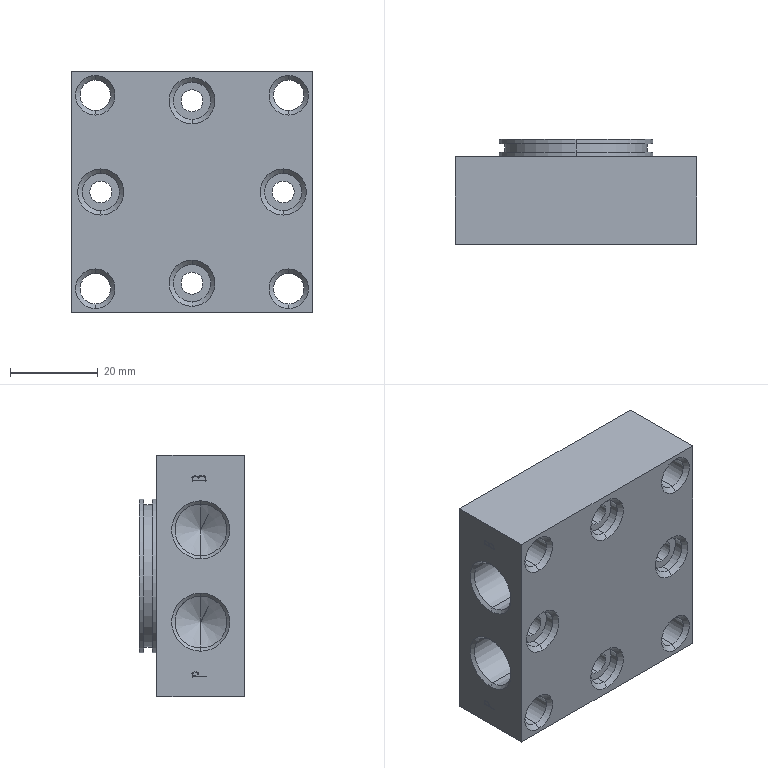Part | SolidWorks | features ICE 7, MirrorPattern 4, Chamfer 2, CirPattern 2, HoleWzd 2, Extrusion 1, RefAxis 1, RevCut 1 | 1 solid | 183 faces | box 55 x 24 x 55 mm | volume 48104 mm3 | plane 63 | cylinder 50 | spline 38 | cone 32 | commonest cylinder face diameters 11.8 x10 4 x8 5 x8 7 x8 8.5 x8 35 x4